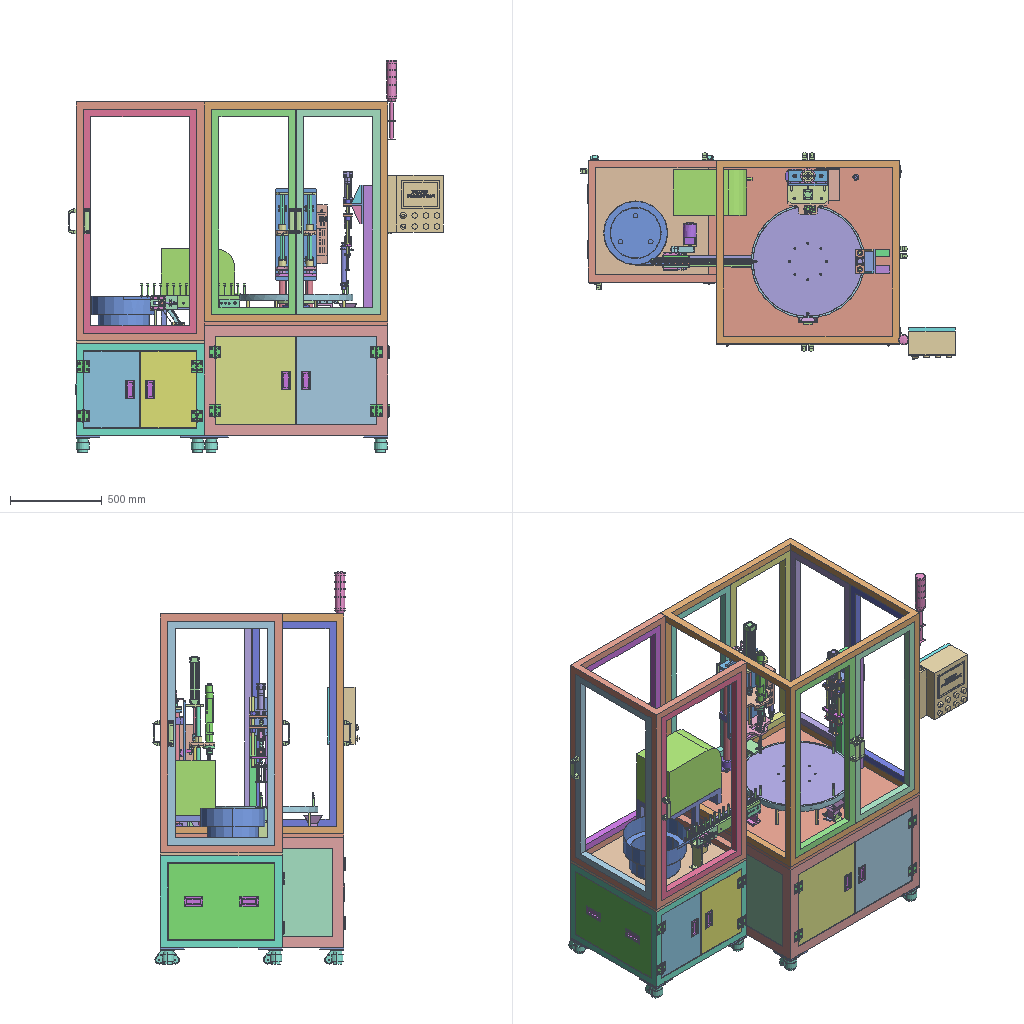Assembly | STEP file | 131 different items | 339 placed | box 2046 x 1125 x 2139 mm
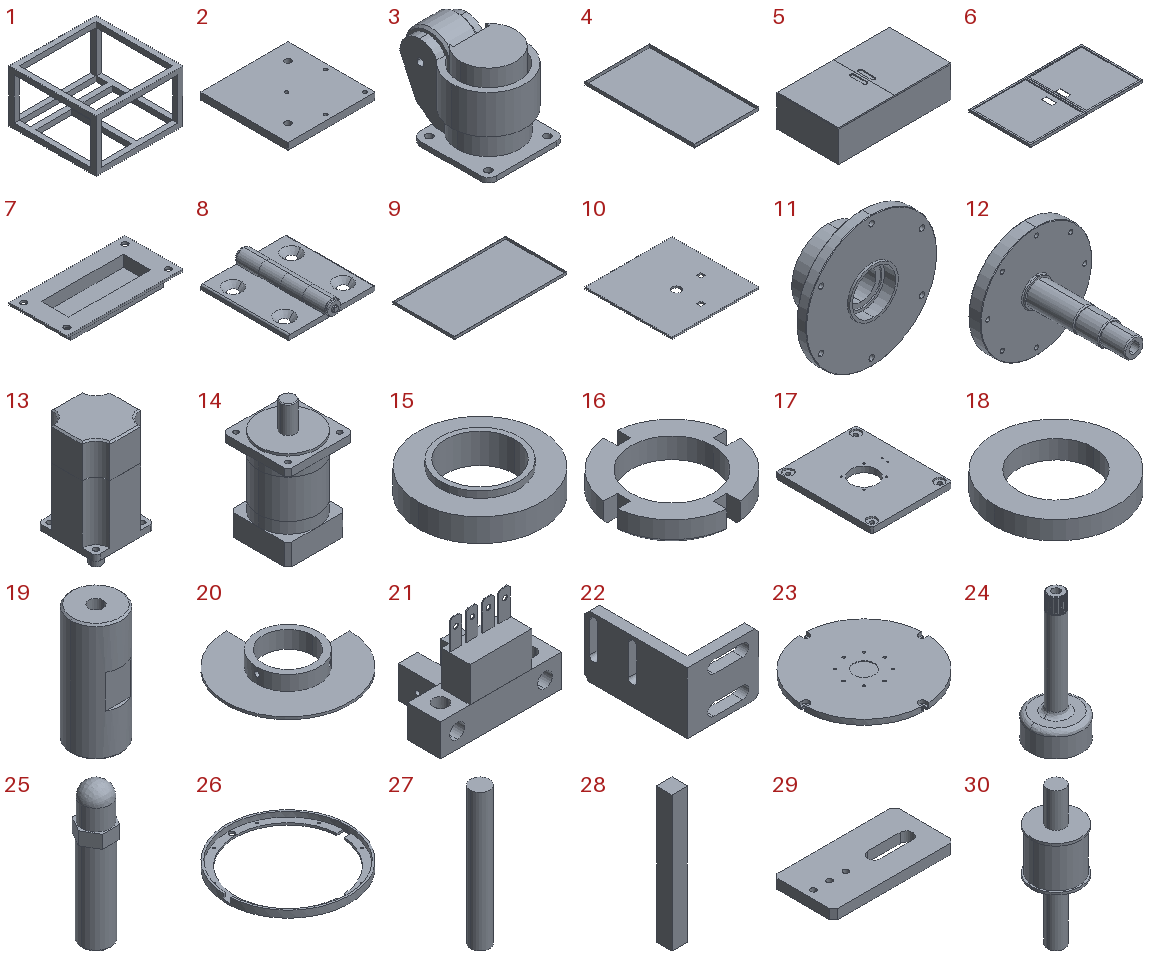Parts list (item | name | quantity | parent item | size | volume):
1 | Lower frame | x1 | in Lower support frame | 1000 x 1000 x 600 mm | 39635953 mm3
2 | Foot plate 2 | x8 | in Lower support frame, Automatic feeding frame | 130 x 130 x 10 mm | 166922 mm3
3 | FM wheel (3 inch) | x8 | in Lower support frame, Automatic feeding frame | 74 x 103.967 x 80 mm | 304180 mm3
4 | Lower sealing plate | x2 | in Lower support frame | 410 x 690 x 20 mm | 485234 mm3
5 | Electrical control box | x1 | in Lower support frame | 880 x 480 x 250 mm | 105113730 mm3
6 | Door | x2 | in Lower support frame | 880 x 480 x 20 mm | 1033932 mm3
7 | Hidden handle | x10 | in Lower support frame, Automatic feeding frame | 102 x 51 x 12.2 mm | 23536 mm3
8 | HHPSN8 hinge | x12 | in Lower support frame, Automatic feeding frame | - | -
9 | Sealing plate | x1 | in Lower support frame | 880 x 480 x 20 mm | 942432 mm3
10 | Large table plate | x1 | in Final assembly | 1000 x 1000 x 20 mm | 19742920 mm3
11 | BB013A02M-04-01A | x1 | in BB013A02M-04-00A | 270 x 95 x 270 mm | 1984635 mm3
12 | BB013A02M-04-02A | x1 | in BB013A02M-04-00A | 230 x 230 x 230 mm | 1390467 mm3
13 | 1FL40-44-0AF21-0AA0 | x1 | in Reducer 2012-6-19 | 80 x 80 x 173 mm | 725829 mm3
14 | PL80-40 | x1 | in Reducer 2012-6-19 | 90 x 90 x 162 mm | 688452 mm3
15 | 30210 | x2 | in BB013A02M-04-00A | 90 x 90 x 21.75 mm | 77564 mm3
16 | M42 nut | x2 | in BB013A02M-04-00A | 71.554 x 71.554 x 12 mm | 23720 mm3
17 | BB013A02M-04-08A | x1 | in BB013A02M-04-00A | 250 x 300 x 18 mm | 1235355 mm3
18 | BB013A02M-04-37A | x1 | in BB013A02M-04-00A | 80 x 80 x 12 mm | 37690 mm3
19 | BB013A02M-04-38A | x4 | in BB013A02M-04-00A | 30 x 30 x 70 mm | 45701 mm3
20 | BB013A02M-04-39A | x1 | in BB013A02M-04-00A | 100 x 100 x 14 mm | 18593 mm3
21 | EE-SX671 (sensing SENSORS) | x1 | in BB013A02M-04-00A | 26.2 x 15.5 x 20.7 mm | 2220 mm3
22 | BB013A02M-04-40A | x1 | in BB013A02M-04-00A | 35 x 50 x 30 mm | 10112 mm3
23 | Turntable | x1 | in Final assembly | 599.815 x 599.815 x 25 mm | 6952769 mm3
24 | Product lower | x20 | in Final assembly, Belt line | 34 x 34 x 83.5 mm | 10000 mm3
25 | Product upper | x3 | in Final assembly | 8.083 x 7 x 31.87 mm | 1117 mm3
26 | Stopper bar | x1 | in Final assembly | 620 x 620 x 35 mm | 1244834 mm3
27 | Support rod | x8 | in Final assembly | 16 x 16 x 114.75 mm | 23072 mm3
28 | Profile | x1 | in Belt line | 40 x 40 x 350 mm | 560000 mm3
29 | Roller fixing plate | x1 | in Belt line | 150 x 75 x 12 mm | 121835 mm3
30 | Driving wheel | x1 | in Belt line | 43 x 43 x 122 mm | 64436 mm3
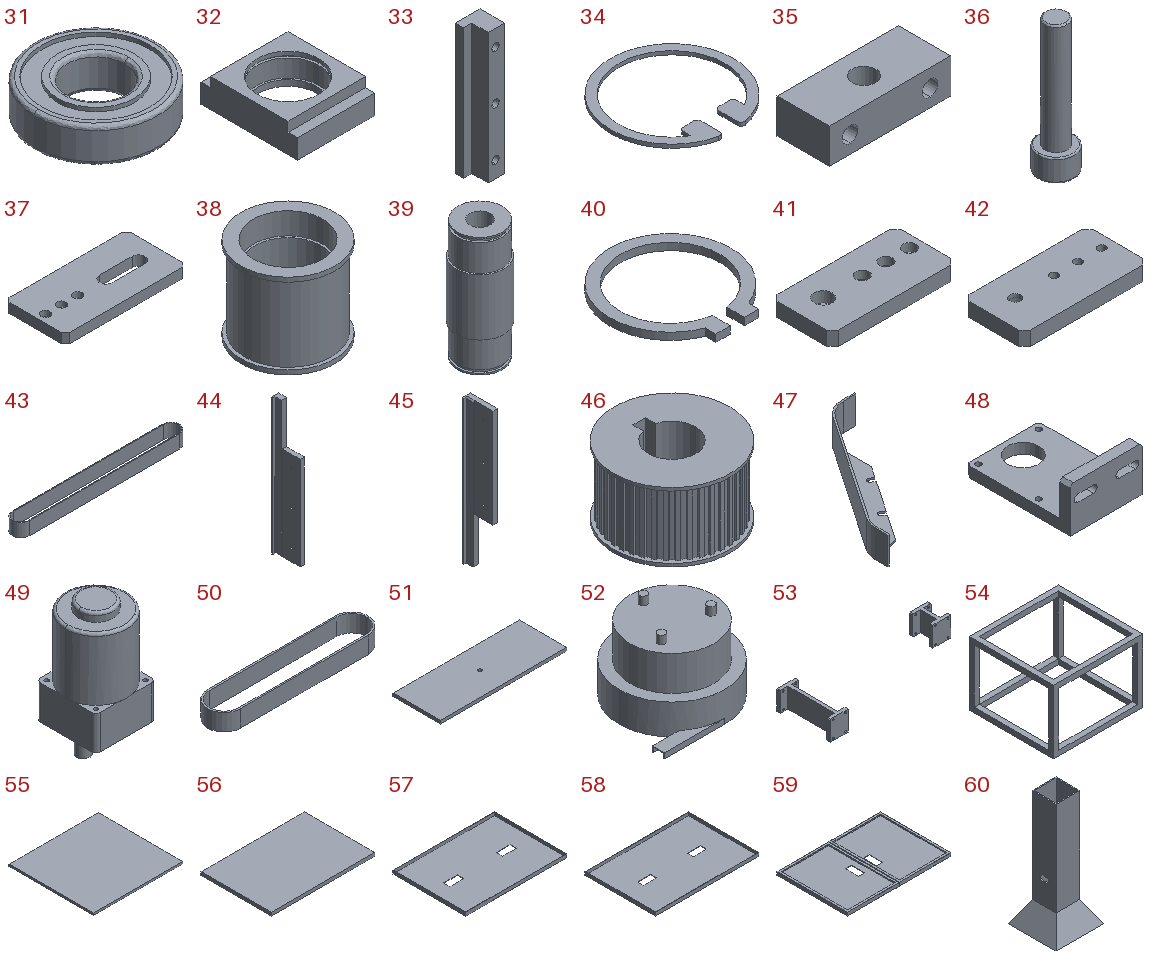31 | 6002 | x4 | in Belt line | 32 x 32 x 9 mm | 4982 mm3
32 | Bearing fixing seat | x2 | in Belt line | 40 x 50 x 15 mm | 16103 mm3
33 | Guide block | x4 | in Belt line | 15 x 15 x 80 mm | 12810 mm3
34 | Inner clip | x2 | in Belt line | 34.4 x 34.017 x 1 mm | 270.275 mm3
35 | Adjusting block | x2 | in Belt line | 35 x 15 x 10 mm | 4094 mm3
36 | Screw | x2 | in Belt line | 13 x 13 x 48 mm | 2788 mm3
37 | Mirror roller fixing plate | x1 | in Belt line | 150 x 75 x 12 mm | 121835 mm3
38 | Driven wheel | x1 | in Belt line | 43 x 43 x 39 mm | 20276 mm3
39 | Driven shaft | x1 | in Belt line | 16 x 16 x 40 mm | 6026 mm3
40 | Outer clip | x2 | in Belt line | 16.8 x 17.727 x 1 mm | 73.853 mm3
41 | Driven wheel fixing plate | x1 | in Belt line | 105 x 52 x 12 mm | 60666 mm3
42 | Mirror driven wheel fixing plate | x1 | in Belt line | 105 x 52 x 12 mm | 60666 mm3
43 | Belt | x1 | in Belt line | 442 x 44 x 35 mm | 64956 mm3
44 | Side stopper bar | x1 | in Belt line | 17.5 x 63 x 335 mm | 183470 mm3
45 | Mirror side stopper bar | x1 | in Belt line | 17.5 x 63 x 335 mm | 183470 mm3
46 | Timing pulley | x2 | in Belt line | 37 x 37 x 22 mm | 16663 mm3
47 | 10020103U05P16_default | x1 | in Belt line | 127 x 167 x 35 mm | 21616 mm3
48 | 10020103U05P11_default | x1 | in Belt line | 70 x 100 x 43 mm | 82196 mm3
49 | M8IA15_default | x1 | in Belt line | 71.8 x 71.8 x 165 mm | 514049 mm3
50 | Timing belt | x1 | in Belt line | 190.16 x 39 x 20 mm | 16742 mm3
51 | Pad plate | x1 | in Belt line | 40 x 15 x 1 mm | 599.215 mm3
52 | Vibratory bowl | x1 | in Belt line | 375 x 350 x 242.5 mm | 663388 mm3
53 | Support plate | x1 | in Belt line | 485 x 170 x 64 mm | 279239 mm3
54 | Small table plate frame | x1 | in Automatic feeding frame | 700 x 665 x 501.75 mm | 10923200 mm3
55 | Small table plate | x1 | in Automatic feeding frame | 700 x 665 x 16 mm | 7448000 mm3
56 | Pad plate 2 | x1 | in Automatic feeding frame | 620 x 420 x 20 mm | 5208000 mm3
57 | Side sealing plate | x1 | in Automatic feeding frame | 585 x 421.75 x 20 mm | 553657 mm3
58 | Rear sealing plate | x1 | in Automatic feeding frame | 620 x 421.75 x 20 mm | 585700 mm3
59 | Side door | x1 | in Automatic feeding frame | 620 x 421.75 x 20 mm | 670167 mm3
60 | Hopper | x2 | in Final assembly | 100 x 100 x 245 mm | 106017 mm3
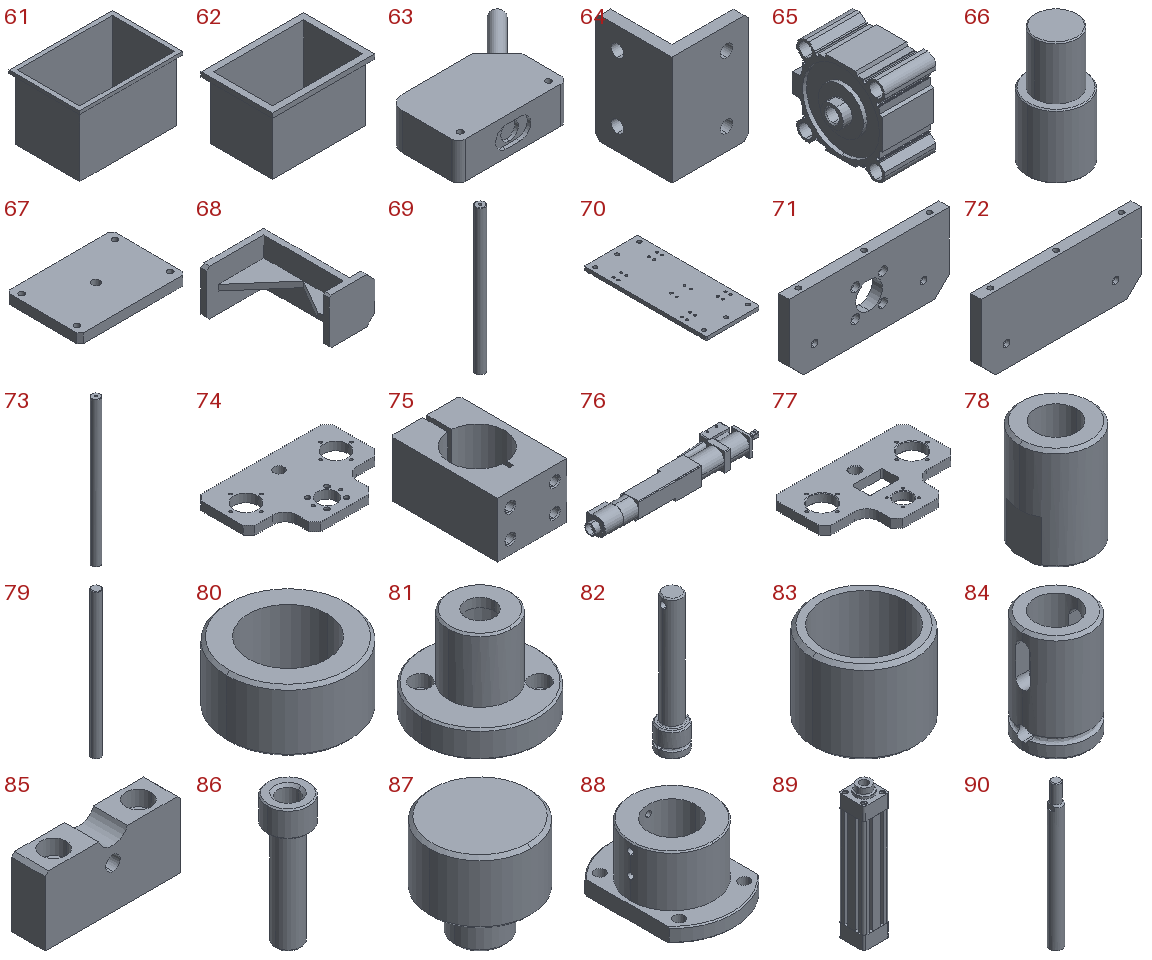61 | Material box | x1 | in Final assembly | 480 x 330 x 300 mm | 3208902 mm3
62 | Material box - copy | x1 | in Final assembly | 330 x 230 x 200 mm | 1493607 mm3
63 | E3Z-T61-L | x4 | in Final assembly | 43.056 x 32.056 x 10.4 mm | 6277 mm3
64 | L bracket | x4 | in Final assembly | 35 x 35 x 50 mm | 15735 mm3
65 | CQ2B100-15DZ(0_0_0) | x1 | in Pressing cylinder | 80 x 123.5 x 117 mm | 628583 mm3
66 | Fixed head | x1 | in Pressing cylinder | 27 x 27 x 55 mm | 25002 mm3
67 | Cylinder pad plate | x1 | in Pressing cylinder | 167 x 117 x 14.75 mm | 282156 mm3
68 | Hook plate | x1 | in Final assembly | 145 x 159.75 x 80 mm | 303088 mm3
69 | fBY02F02M-00-02A | x2 | in fBY02F02M-01-00A | 40 x 40 x 620 mm | 776363 mm3
70 | fBY02F02M-00-04A | x1 | in fBY02F02M-01-00A | 220 x 500 x 14 mm | 1483001 mm3
71 | fBY02F02M-00-08A | x1 | in fBY02F02M-01-00A | 220 x 14 x 100 mm | 276380 mm3
72 | fBY02F02M-00-05A | x1 | in fBY02F02M-01-00A | 220 x 14 x 100 mm | 295677 mm3
73 | fBY02F02M-00-20A | x2 | in fBY02F02M-01-00A | 25 x 25 x 430 mm | 209515 mm3
74 | fBY02F02M-00-07A | x1 | in fBY02F02M-01-00A | 220 x 140 x 14 mm | 291524 mm3
75 | fBY02F02M-00-03A | x4 | in fBY02F02M-01-00A | 50 x 78 x 40 mm | 94734 mm3
76 | fNFT-401RM1A-S | x1 | in fBY02F02M-01-00A | 356.359 x 63.246 x 40.132 mm | 479956 mm3
77 | fBY02F02M-00-06A | x1 | in fBY02F02M-01-00A | 220 x 140 x 14 mm | 261096 mm3
78 | fBY02F02M-00-13A | x1 | in fBY02F02M-01-00A | 25 x 25 x 35 mm | 12210 mm3
79 | fBY02F02M-00-21A | x1 | in fBY02F02M-01-00A | 16 x 16 x 260 mm | 52228 mm3
80 | fBY02F02M-00-19A | x2 | in fBY02F02M-01-00A | 40 x 40 x 20 mm | 14795 mm3
81 | fBY02F02M-00-14A | x1 | in fBY02F02M-02-00A | 65 x 65 x 50 mm | 50405 mm3
82 | fBY02F02M-00-15A | x1 | in fBY02F02M-02-00A | 22 x 22 x 110 mm | 21708 mm3
83 | fBY02F02M-00-16A | x1 | in fBY02F02M-02-00A | 30 x 30 x 24 mm | 7122 mm3
84 | fBY02F02M-00-17A | x1 | in fBY02F02M-02-00A | 24 x 24 x 38 mm | 10216 mm3
85 | fBY02F02M-00-10A | x1 | in fBY02F02M-01-00A | 80 x 20 x 40 mm | 54175 mm3
86 | fBY02F02M-00-11A | x1 | in fBY02F02M-01-00A | 16 x 16 x 50 mm | 4764 mm3
87 | fBY02F02M-00-12A | x1 | in fBY02F02M-01-00A | 16 x 16 x 16 mm | 2297 mm3
88 | fBY02F02M-00-01A | x2 | in fBY02F02M-01-00A | 76 x 104 x 55 mm | 203193 mm3
89 | fA_CP95SB40-150 (0) | x1 | in fcp95sb40-150 | 52 x 52 x 276 mm | 568979 mm3
90 | fA_CP95SB40-150 (0)1 | x1 | in fcp95sb40-150 | 16 x 16 x 188 mm | 35479 mm3
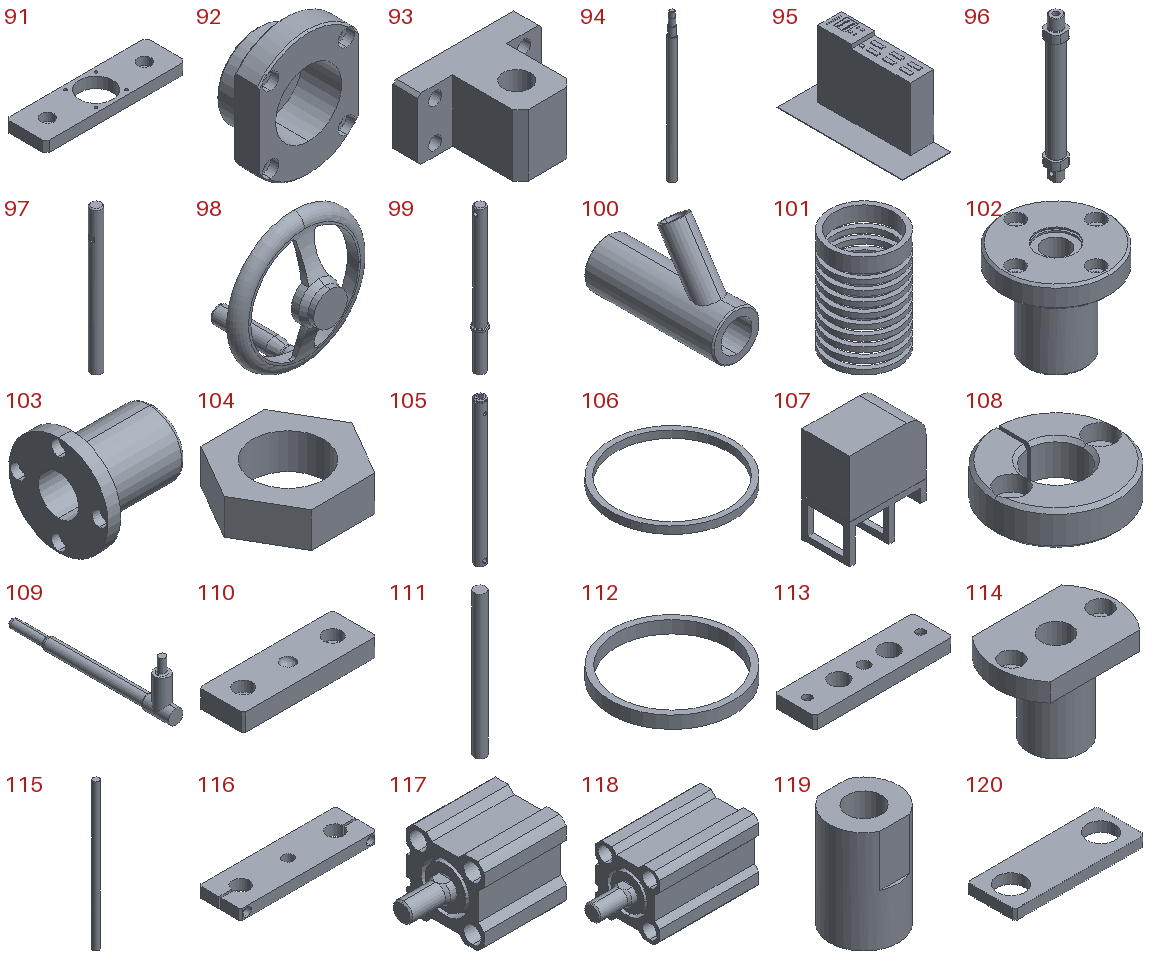91 | fBY02F02M-00-24A | x1 | in fBY02F02M-01-00A | 210 x 60 x 16 mm | 159812 mm3
92 | fBY02F02M-00-25A | x1 | in fBY02F02M-01-00A | 60 x 31 x 75.753 mm | 56251 mm3
93 | fBY02F02M-00-26A | x1 | in fBY02F02M-01-00A | 80 x 60 x 40 mm | 98419 mm3
94 | fBY02F02M-00-27A | x1 | in fBY02F02M-01-00A | 20 x 20 x 409 mm | 120074 mm3
95 | f401kongzhiqi | x1 | in fBY02F02M-01-00A | 122.5 x 320 x 173.5 mm | 2367856 mm3
96 | fA_C85N25-100T(OUT)1 | x1 | in fC85 | 30 x 30 x 257.5 mm | 131255 mm3
97 | fA_C85N25-100T(OUT) | x1 | in fC85 | 10 x 10 x 129 mm | 10086 mm3
98 | fSHLN80 | x1 | in fBY02F02M-01-00A | 80 x 67 x 81.1 mm | 18367 mm3
99 | fBY012F01M-03-01A | x1 | in fBY012F01M-03-00A | 16 x 16 x 172 mm | 18180 mm3
100 | fBY012F01M-03-02A | x1 | in fBY012F01M-03-00A | 18.4 x 50 x 39.602 mm | 7485 mm3
101 | f5-13-063 | x1 | in fBY012F01M-03-00A | 14.1 x 14.1 x 21 mm | 493.858 mm3
102 | fBY02F02M-00-30A | x1 | in fBY02F02M-01-00A | 50 x 50 x 45 mm | 36506 mm3
103 | LHFR-N25 | x4 | in fBY02F02M-01-00A | 59 x 62 x 62 mm | 57510 mm3
104 | M16 nut | x1 | in fBY02F02M-01-00A | 28.868 x 25 x 8 mm | 2722 mm3
105 | Rotating rod | x1 | in fBY02F02M-01-00A | 12 x 12 x 172 mm | 18082 mm3
106 | Extension spring | x25 | in fBY02F02M-01-00A | 17 x 17 x 1 mm | 38.288 mm3
107 | Screw feeder | x1 | in Final assembly | 430 x 250 x 502.25 mm | 31721317 mm3
108 | 08 displacement fixing | x3 | in Displacement detection height | 18 x 17.971 x 5 mm | 899.318 mm3
109 | 08 displacement_default | x1 | in Displacement detection height | 10 x 114.88 x 37 mm | 7298 mm3
110 | Displacement press plate | x1 | in Displacement detection height | 60 x 20 x 8 mm | 8957 mm3
111 | Displacement buffer guide | x2 | in Displacement detection height | 8 x 8 x 100 mm | 5027 mm3
112 | Small spring | x70 | in Displacement detection height | 10 x 10 x 1 mm | 14.923 mm3
113 | Probe fixing plate | x1 | in Displacement detection height | 110 x 32 x 10 mm | 29438 mm3
114 | LMH8UU | x2 | in Displacement detection height | 32 x 21 x 24 mm | 5030 mm3
115 | Guide shaft | x2 | in Displacement detection height | 16 x 16 x 380 mm | 76404 mm3
116 | Cylinder fixing plate 1 | x1 | in Displacement detection height | 130 x 40 x 10 mm | 45360 mm3
117 | CQ2B25-20DM(0_0_0) | x1 | in Displacement detection height | - | -
118 | CQ2B25-40DM(0_0_0) | x1 | in Displacement detection height | - | -
119 | Cylinder joint | x1 | in Displacement detection height | 20 x 20 x 30 mm | 6892 mm3
120 | Linear support fixing plate | x2 | in Displacement detection height | 130 x 48 x 10 mm | 50005 mm3
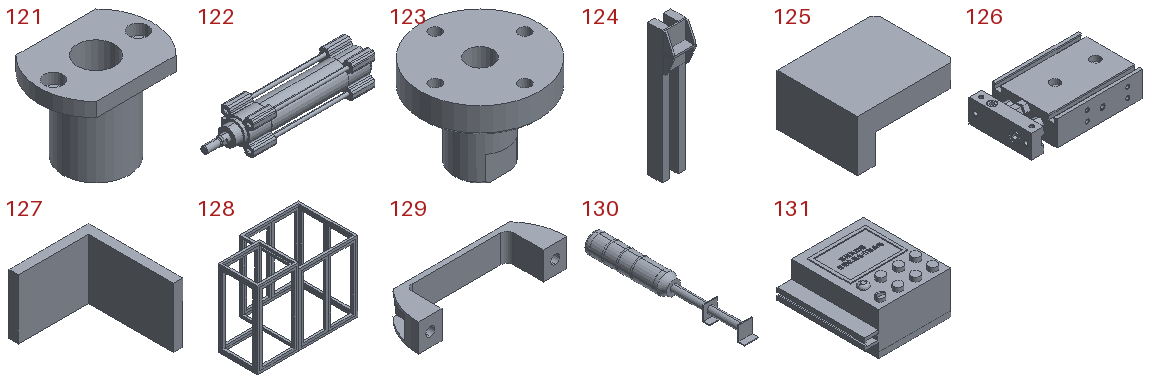121 | LMH16UU | x4 | in Displacement detection height | 48 x 34 x 37 mm | 20039 mm3
122 | C96SB32-80(0_0_0) | x1 | in Displacement detection height | - | -
123 | Connector | x1 | in Displacement detection height | 45 x 45 x 35 mm | 19325 mm3
124 | Connecting plate | x1 | in Displacement detection height | 130 x 142.1 x 745 mm | 5233440 mm3
125 | Cutting plate | x1 | in Cutting mechanism | 44 x 36 x 23 mm | 19544 mm3
126 | CXSM20-35(0_0_0) | x1 | in Cutting mechanism | - | -
127 | Cylinder support plate | x1 | in Cutting mechanism | 85 x 100.75 x 64 mm | 112480 mm3
128 | Upper frame | x1 | in Final assembly | 1700 x 1000 x 1302 mm | 80127840 mm3
129 | UPCN26-B plastic handle | x9 | in Final assembly | 139 x 41 x 26 mm | 36631 mm3
130 | Alarm light 3 | x1 | in Final assembly | 56 x 452 x 56 mm | 602047 mm3
131 | Touch screen 2 | x1 | in Final assembly | 305 x 310 x 172 mm | 12316127 mm3
Placements (level | parent | child | x y z in mm | rotation matrix by rows), first 300 of 352 lines:
1 | Final assembly | Lower support frame | -11.646 -4.778 45.0 | 1 0 0 0 1 0 0 0 1
2 | Lower support frame | Lower frame | -455.325 382.615 -250.0 | 1 0 0 0 1 0 0 0 1
2 | Lower support frame | Foot plate 2 | -452.697 -567.103 -260.0 | 0 1 0 -1 0 0 0 0 1
2 | Lower support frame | Foot plate 2 | -452.697 302.897 -260.0 | 0 1 0 -1 0 0 0 0 1
2 | Lower support frame | Foot plate 2 | 417.303 -567.103 -260.0 | 0 1 0 -1 0 0 0 0 1
2 | Lower support frame | Foot plate 2 | 417.303 302.897 -260.0 | 0 1 0 -1 0 0 0 0 1
2 | Lower support frame | FM wheel (3 inch) | -448.325 -550.385 -260.0 | -1 0 0 0 1 0 0 0 -1
2 | Lower support frame | FM wheel (3 inch) | -448.325 375.615 -260.0 | 1 0 0 0 -1 0 0 0 -1
2 | Lower support frame | FM wheel (3 inch) | 477.675 -550.385 -260.0 | -1 0 0 0 1 0 0 0 -1
2 | Lower support frame | FM wheel (3 inch) | 477.675 375.615 -260.0 | 1 0 0 0 -1 0 0 0 -1
2 | Lower support frame | Lower sealing plate | 249.61 -182.385 -190.0 | -1 0 0 0 1 0 0 0 -1
2 | Lower support frame | Electrical control box | 14.675 162.615 50.0 | 1 0 0 0 0 1 0 -1 0
2 | Lower support frame | Lower sealing plate | -220.33 -182.385 -190.0 | -1 0 0 0 1 0 0 0 -1
2 | Lower support frame | Door | 514.675 -87.385 50.0 | 0 0 -1 -1 0 0 0 1 0
2 | Lower support frame | Hidden handle | 504.475 -32.885 50.0 | 0 0 1 0 1 0 -1 0 0
2 | Lower support frame | Hidden handle | 504.475 -141.885 50.0 | 0 0 1 0 1 0 -1 0 0
2 | Lower support frame | HHPSN8 hinge | 520.175 352.615 205.3 | 0 0 1 -1 0 0 0 -1 0
2 | Lower support frame | HHPSN8 hinge | 520.175 352.615 -114.7 | 0 0 1 -1 0 0 0 -1 0
2 | Lower support frame | HHPSN8 hinge | 520.175 -527.385 205.3 | 0 0 1 -1 0 0 0 -1 0
2 | Lower support frame | HHPSN8 hinge | 520.175 -527.385 -114.7 | 0 0 1 -1 0 0 0 -1 0
2 | Lower support frame | HHPSN8 hinge | 454.675 -592.885 205.3 | -1 0 0 0 0 -1 0 -1 0
2 | Lower support frame | HHPSN8 hinge | 454.675 -592.885 -114.7 | -1 0 0 0 0 -1 0 -1 0
2 | Lower support frame | Hidden handle | 69.175 -577.185 50.0 | 0 1 0 0 0 -1 -1 0 0
2 | Lower support frame | Hidden handle | -39.825 -577.185 50.0 | 0 1 0 0 0 -1 -1 0 0
2 | Lower support frame | HHPSN8 hinge | -425.325 -592.885 -114.7 | -1 0 0 0 0 -1 0 -1 0
2 | Lower support frame | HHPSN8 hinge | -425.325 -592.885 205.3 | -1 0 0 0 0 -1 0 -1 0
2 | Lower support frame | Door | 14.675 -587.385 50.0 | -1 0 0 0 0 1 0 1 0
2 | Lower support frame | Sealing plate | -485.325 -87.385 50.0 | 0 0 1 1 0 0 0 1 0
1 | Final assembly | Large table plate | 3.029 -92.163 395.0 | 1 0 0 0 1 0 0 0 1
1 | Final assembly | BB013A02M-04-00A | 344.4 -189.063 134.949 | 1 0 0 0 1 0 0 0 1
2 | BB013A02M-04-00A | BB013A02M-04-01A | -341.371 46.9 211.718 | 0.9983 0 0.05751 0.05751 0 -0.9983 0 1 0
2 | BB013A02M-04-00A | BB013A02M-04-02A | -341.371 46.9 172.801 | 1 0 0 0 0 -1 0 1 0
2 | BB013A02M-04-00A | Reducer 2012-6-19 | -343.105 58.644 3.551 | 0 1 0 1 0 0 0 0 -1
3 | Reducer 2012-6-19 | 1FL40-44-0AF21-0AA0 | -11.745 1.734 -46.5 | 1 0 0 0 1 0 0 0 1
3 | Reducer 2012-6-19 | PL80-40 | -11.745 1.734 -46.5 | 1 0 0 0 -1 0 0 0 -1
2 | BB013A02M-04-00A | 30210 | -341.371 46.9 353.051 | 1 0 0 0 1 0 0 0 1
2 | BB013A02M-04-00A | 30210 | -341.371 46.9 298.051 | -0.9237 -0.383 0 -0.383 0.9237 0 0 0 -1
2 | BB013A02M-04-00A | M42 nut | -341.371 46.9 252.301 | 0.9998 0.01986 0 -0.01986 0.9998 0 0 0 1
2 | BB013A02M-04-00A | M42 nut | -341.371 46.9 240.301 | 0.9998 0.01986 0 -0.01986 0.9998 0 0 0 1
2 | BB013A02M-04-00A | BB013A02M-04-08A | -341.371 46.9 172.051 | 1 0 0 0 1 0 0 0 1
2 | BB013A02M-04-00A | BB013A02M-04-37A | -341.371 46.9 264.301 | 1 0 0 0 1 0 0 0 1
2 | BB013A02M-04-00A | BB013A02M-04-38A | -446.371 -83.1 260.051 | -0.9237 -0.383 0 -0.383 0.9237 0 0 0 -1
2 | BB013A02M-04-00A | BB013A02M-04-38A | -446.371 176.899 260.051 | -0.9237 -0.383 0 -0.383 0.9237 0 0 0 -1
2 | BB013A02M-04-00A | BB013A02M-04-38A | -236.371 -83.1 260.051 | -0.9237 -0.383 0 -0.383 0.9237 0 0 0 -1
2 | BB013A02M-04-00A | BB013A02M-04-38A | -236.371 176.899 260.051 | -0.9237 -0.383 0 -0.383 0.9237 0 0 0 -1
2 | BB013A02M-04-00A | BB013A02M-04-39A | -341.371 46.9 227.801 | 1 0 0 0 -1 0 0 0 -1
2 | BB013A02M-04-00A | EE-SX671 (sensing SENSORS) | -281.371 47.374 226.301 | 0 -1 0 0 0 1 -1 0 0
2 | BB013A02M-04-00A | BB013A02M-04-40A | -281.371 73.9 240.051 | 1 0 0 0 0 -1 0 1 0
1 | Final assembly | Turntable | 3.029 -142.163 564.75 | -1 0 0 0 1 0 0 0 -1
1 | Final assembly | Product lower | 3.029 -425.163 539.75 | 0 -1 0 1 0 0 0 0 1
1 | Final assembly | Product lower | -279.971 -142.163 539.75 | 1 0 0 0 1 0 0 0 1
1 | Final assembly | Product lower | 3.029 140.837 539.75 | 0 1 0 -1 0 0 0 0 1
1 | Final assembly | Product lower | 286.029 -142.163 539.75 | -1 0 0 0 -1 0 0 0 1
1 | Final assembly | Product upper | 3.029 140.837 632.25 | 1 0 0 0 1 0 0 0 1
1 | Final assembly | Product upper | 286.029 -142.163 632.25 | 0 1 0 -1 0 0 0 0 1
1 | Final assembly | Product upper | 3.029 -425.163 632.25 | -1 0 0 0 -1 0 0 0 1
1 | Final assembly | Stopper bar | 3.029 -142.163 529.75 | 1 0 0 0 1 0 0 0 1
1 | Final assembly | Support rod | -260.203 -33.129 415.0 | 1 0 0 0 1 0 0 0 1
1 | Final assembly | Support rod | -260.203 -251.197 415.0 | 0.7071 -0.7071 0 0.7071 0.7071 0 0 0 1
1 | Final assembly | Support rod | -106.005 -405.395 415.0 | 0 -1 0 1 0 0 0 0 1
1 | Final assembly | Support rod | 112.063 -405.395 415.0 | -0.7071 -0.7071 0 0.7071 -0.7071 0 0 0 1
1 | Final assembly | Support rod | 266.261 -251.197 415.0 | -1 0 0 0 -1 0 0 0 1
1 | Final assembly | Support rod | 266.261 -33.129 415.0 | -0.7071 0.7071 0 -0.7071 -0.7071 0 0 0 1
1 | Final assembly | Support rod | 112.063 121.069 415.0 | 0 1 0 -1 0 0 0 0 1
1 | Final assembly | Support rod | -106.005 121.069 415.0 | 0.7071 0.7071 0 -0.7071 0.7071 0 0 0 1
1 | Final assembly | Belt line | -601.971 -91.057 499.385 | 0 0 -1 -1 0 0 0 1 0
2 | Belt line | Profile | 51.106 18.365 -250.0 | 1 0 0 0 1 0 0 0 1
2 | Belt line | Roller fixing plate | 83.106 20.865 115.0 | 0 0 -1 0 1 0 1 0 -0
2 | Belt line | Driving wheel | 33.606 18.365 125.0 | 0 0 1 0.7219 0.692 0 -0.692 0.7219 0
2 | Belt line | 6002 | 95.106 18.365 125.0 | 0 0 -1 -0.5396 0.8419 0 0.8419 0.5396 0
2 | Belt line | Bearing fixing seat | 83.106 18.365 125.0 | 0 0 1 0 1 0 -1 0 0
2 | Belt line | Guide block | 93.106 -1.635 105.0 | 0 1 0 -1 0 0 0 0 1
2 | Belt line | Guide block | 93.106 38.365 185.0 | 0 1 0 1 0 0 0 0 -1
2 | Belt line | Inner clip | 96.106 18.365 125.0 | 0 0 -1 0 1 0 1 0 -0
2 | Belt line | Adjusting block | 90.606 18.365 75.0 | 0 1 0 -1 0 0 0 0 1
2 | Belt line | Screw | 90.606 18.365 57.0 | 1 0 0 0 1 0 0 0 1
2 | Belt line | Mirror roller fixing plate | 19.106 20.865 115.0 | 0 0 -1 0 1 0 1 0 -0
2 | Belt line | Guide block | 9.106 38.365 105.0 | 0 -1 0 1 0 0 0 0 1
2 | Belt line | Bearing fixing seat | 19.106 18.365 125.0 | 0 0 -1 0 1 0 1 0 0
2 | Belt line | 6002 | 7.106 18.365 125.0 | 0 0 1 0.5396 0.8419 0 -0.8419 0.5396 0
2 | Belt line | Inner clip | 7.106 18.365 125.0 | 0 0 -1 0 1 0 1 0 0
2 | Belt line | Screw | 11.606 18.365 57.0 | 1 0 0 0 1 0 0 0 1
2 | Belt line | Adjusting block | 11.606 18.365 75.0 | 0 -1 0 1 0 0 0 0 1
2 | Belt line | Guide block | 9.106 -1.635 185.0 | 0 -1 0 -1 0 0 0 0 -1
2 | Belt line | Driven wheel | 68.606 18.365 -273.0 | 0 0 -1 0 1 0 1 0 0
2 | Belt line | 6002 | 69.606 18.365 -273.0 | 0 0 -1 0 1 0 1 0 0
2 | Belt line | 6002 | 41.606 18.365 -273.0 | 0 0 -1 0 1 0 1 0 0
2 | Belt line | Driven shaft | 60.606 18.365 -273.0 | 0 0 -1 0 1 0 1 0 0
2 | Belt line | Outer clip | 70.606 18.365 -273.0 | 0 0 -1 0 1 0 1 0 0
2 | Belt line | Outer clip | 32.606 18.365 -273.0 | 0 0 -1 0 1 0 1 0 0
2 | Belt line | Driven wheel fixing plate | 31.106 23.365 -242.5 | 0 0 -1 0 1 0 1 0 -0
2 | Belt line | Mirror driven wheel fixing plate | 71.106 23.365 -242.5 | 0 0 -1 0 1 0 1 0 -0
2 | Belt line | Belt | 68.606 18.365 -273.0 | 0 0 -1 0 1 0 1 0 -0
2 | Belt line | Side stopper bar | 31.106 -3.635 40.0 | -1 0 0 0 1 0 0 0 -1
2 | Belt line | Mirror side stopper bar | 71.106 -3.635 40.0 | 1 0 0 0 1 0 0 0 1
2 | Belt line | Timing pulley | -19.894 18.365 125.0 | 0 0 1 0 1 0 -1 0 0
2 | Belt line | 10020103U05P16_default | 2.106 18.365 125.0 | 0 0 -1 0 1 0 1 0 -0
2 | Belt line | Timing pulley | 0.1063 -106.635 40.0 | 0 0 -1 0 1 0 1 0 -0
2 | Belt line | 10020103U05P11_default | -30.894 -136.635 40.0 | 0 0 -1 0 1 0 1 0 -0
2 | Belt line | M8IA15_default | -40.894 -121.635 40.0 | 0 0 -1 0 1 0 1 0 0
2 | Belt line | Timing belt | -19.894 18.365 125.0 | 0 0 1 -0.8269 0.5623 0 -0.5623 -0.8269 0
2 | Belt line | Pad plate | 51.106 40.365 -287.5 | 1 0 0 0 0 -1 0 1 0
2 | Belt line | Product lower | 51.106 40.365 -287.5 | 1 0 0 0 0 1 0 -1 0
2 | Belt line | Product lower | 51.106 40.365 -252.5 | 1 0 0 0 0 1 0 -1 0
2 | Belt line | Product lower | 51.106 40.365 -217.5 | 1 0 0 0 0 1 0 -1 0
2 | Belt line | Product lower | 51.106 40.365 -182.5 | 1 0 0 0 0 1 0 -1 0
2 | Belt line | Product lower | 51.106 40.365 -147.5 | 1 0 0 0 0 1 0 -1 0
2 | Belt line | Product lower | 51.106 40.365 -112.5 | 1 0 0 0 0 1 0 -1 0
2 | Belt line | Product lower | 51.106 40.365 -77.5 | 1 0 0 0 0 1 0 -1 0
2 | Belt line | Product lower | 51.106 40.365 -42.5 | 1 0 0 0 0 1 0 -1 0
2 | Belt line | Product lower | 51.106 40.365 -7.5 | 1 0 0 0 0 1 0 -1 0
2 | Belt line | Product lower | 51.106 40.365 27.5 | 1 0 0 0 0 1 0 -1 0
2 | Belt line | Product lower | 51.106 40.365 62.5 | 1 0 0 0 0 1 0 -1 0
2 | Belt line | Product lower | 51.106 40.365 97.5 | 1 0 0 0 0 1 0 -1 0
2 | Belt line | Product lower | 51.106 40.365 132.5 | 1 0 0 0 0 1 0 -1 0
2 | Belt line | Vibratory bowl | -103.894 55.865 335.0 | 0 -1 0 0 0 -1 1 0 -0
2 | Belt line | Product lower | 51.106 40.365 167.5 | 1 0 0 0 0 1 0 -1 0
2 | Belt line | Product lower | 51.106 40.365 202.5 | 1 0 0 0 0 1 0 -1 0
2 | Belt line | Product lower | 51.106 40.365 237.5 | 1 0 0 0 0 1 0 -1 0
2 | Belt line | Support plate | 19.106 -11.635 190.0 | 0 0 1 0 1 0 -1 0 0
1 | Final assembly | Automatic feeding frame | -852.986 77.278 45.875 | 1 0 0 0 1 0 0 0 1
2 | Automatic feeding frame | Small table plate frame | 6.015 -1.941 -250.875 | 1 0 0 0 1 0 0 0 1
2 | Automatic feeding frame | Small table plate | 6.015 -1.941 250.875 | 1 0 0 0 1 0 0 0 1
2 | Automatic feeding frame | Foot plate 2 | -311.357 -314.159 -260.875 | 0 1 0 -1 0 0 0 0 1
2 | Automatic feeding frame | Foot plate 2 | -311.357 220.841 -260.875 | 0 1 0 -1 0 0 0 0 1
2 | Automatic feeding frame | Foot plate 2 | 258.643 -314.159 -260.875 | 0 1 0 -1 0 0 0 0 1
2 | Automatic feeding frame | Foot plate 2 | 258.643 220.841 -260.875 | 0 1 0 -1 0 0 0 0 1
2 | Automatic feeding frame | FM wheel (3 inch) | -306.985 -297.441 -260.875 | -1 0 0 0 1 0 0 0 -1
2 | Automatic feeding frame | FM wheel (3 inch) | -306.985 293.559 -260.875 | -1 0 0 0 1 0 0 0 -1
2 | Automatic feeding frame | FM wheel (3 inch) | 319.015 -297.441 -260.875 | -1 0 0 0 1 0 0 0 -1
2 | Automatic feeding frame | FM wheel (3 inch) | 319.015 293.559 -260.875 | -1 0 0 0 1 0 0 0 -1
2 | Automatic feeding frame | Pad plate 2 | 6.015 80.559 -230.875 | 1 0 0 0 1 0 0 0 1
2 | Automatic feeding frame | Side sealing plate | -343.985 -1.941 -0.0 | 0 0 1 1 0 0 0 1 0
2 | Automatic feeding frame | Hidden handle | -333.785 150.059 -0.0 | 0 0 -1 -1 0 0 0 1 -0
2 | Automatic feeding frame | Rear sealing plate | 6.015 330.559 0.0 | 1 0 0 0 0 -1 0 1 0
2 | Automatic feeding frame | Hidden handle | 155.515 320.359 0.0 | 1 0 0 0 0 1 0 -1 0
2 | Automatic feeding frame | Hidden handle | -143.485 320.359 0.0 | 1 0 0 0 0 1 0 -1 0
2 | Automatic feeding frame | Side door | 6.015 -334.441 -0.0 | 1 0 0 0 0 1 0 -1 0
2 | Automatic feeding frame | Hidden handle | 60.515 -324.241 0.0 | 0 -1 0 0 0 -1 1 0 0
2 | Automatic feeding frame | Hidden handle | -48.485 -324.241 0.0 | 0 -1 0 0 0 -1 1 0 0
2 | Automatic feeding frame | HHPSN8 hinge | 316.015 -339.941 126.175 | 1 0 0 0 0 -1 0 1 0
2 | Automatic feeding frame | HHPSN8 hinge | 316.015 -339.941 -143.825 | 1 0 0 0 0 -1 0 1 0
2 | Automatic feeding frame | HHPSN8 hinge | -303.985 -339.941 126.175 | 1 0 0 0 0 -1 0 1 0
2 | Automatic feeding frame | HHPSN8 hinge | -303.985 -339.941 -143.825 | 1 0 0 0 0 -1 0 1 0
2 | Automatic feeding frame | Hidden handle | -333.785 -153.941 -0.0 | 0 0 -1 -1 0 0 0 1 -0
1 | Final assembly | Hopper | 3.029 -425.163 514.75 | -1 0 0 0 1 0 0 0 -1
1 | Final assembly | Hopper | 286.029 -142.163 514.75 | 0 -1 0 -1 0 0 0 0 -1
1 | Final assembly | Material box | -36.971 -390.163 -145.0 | 1 0 0 0 1 0 0 0 1
1 | Final assembly | Material box - copy | 306.029 -142.163 -145.0 | 0 -1 0 1 0 0 0 0 1
1 | Final assembly | E3Z-T61-L | -21.971 -442.163 415.0 | 0 -1 0 1 0 0 0 0 1
1 | Final assembly | E3Z-T61-L | 28.029 -442.163 425.4 | 0 1 0 1 0 0 0 0 -1
1 | Final assembly | E3Z-T61-L | 303.029 -117.163 425.4 | -1 0 0 0 1 0 0 0 -1
1 | Final assembly | E3Z-T61-L | 303.029 -167.163 415.0 | -1 0 0 0 -1 0 0 0 1
1 | Final assembly | L bracket | 28.029 -450.163 450.0 | 0 0 -1 -1 0 0 0 1 0
1 | Final assembly | L bracket | -21.971 -400.163 450.0 | 0 0 1 1 0 0 0 1 0
1 | Final assembly | L bracket | 261.029 -167.163 450.0 | -1 0 0 0 0 1 0 1 0
1 | Final assembly | L bracket | 311.029 -117.163 450.0 | 1 0 0 0 0 -1 0 1 0
1 | Final assembly | Pressing cylinder | 22.325 140.837 460.834 | 0 -1 0 0 0 1 -1 0 0
2 | Pressing cylinder | CQ2B100-15DZ(0_0_0) | -36.916 19.296 -0.0 | 1 0 0 0 1 0 0 0 1
2 | Pressing cylinder | Fixed head | -78.916 19.296 0.0 | 0 0 1 0 1 0 -1 0 -0
2 | Pressing cylinder | Cylinder pad plate | 45.834 19.296 -0.0 | 0 0 -1 -1 0 0 0 1 0
1 | Final assembly | Hook plate | -36.971 147.837 564.75 | 0 0 1 1 0 0 0 1 -0
1 | Final assembly | fBY02F02M-01-00A | -179.249 533.293 824.53 | 0 1 -0.000385 -1 0 0 0 0.000385 1
2 | fBY02F02M-01-00A | fBY02F02M-00-02A | 210.454 109.802 -397.719 | 0.4882 -0.8727 0 0.8727 0.4882 0 0 0 1
2 | fBY02F02M-01-00A | fBY02F02M-00-02A | 210.454 254.802 -397.719 | 0.9253 0.3793 0 -0.3793 0.9253 0 0 0 1
2 | fBY02F02M-01-00A | fBY02F02M-00-04A | 264.454 292.302 318.281 | 0 0 -1 -1 0 0 0 1 0
2 | fBY02F02M-01-00A | fBY02F02M-00-08A | 362.454 292.302 298.281 | 0 0 -1 -1 0 0 0 1 0
2 | fBY02F02M-01-00A | fBY02F02M-00-05A | 362.454 292.302 -145.719 | 0 0 -1 -1 0 0 0 1 0
2 | fBY02F02M-01-00A | fBY02F02M-00-20A | 332.454 107.302 -145.719 | 1 0 0 0 1 0 0 0 1
2 | fBY02F02M-01-00A | fBY02F02M-00-20A | 332.454 257.302 -145.719 | 0.9995 0.03267 0 -0.03267 0.9995 0 0 0 1
2 | fBY02F02M-01-00A | fBY02F02M-00-07A | 282.454 292.302 86.584 | 0 -1 0 -1 0 0 0 0 -1
2 | fBY02F02M-01-00A | fBY02F02M-00-03A | 250.454 254.802 -71.719 | 0 -1 0 1 0 0 0 0 1
2 | fBY02F02M-01-00A | fBY02F02M-00-03A | 250.454 254.802 208.281 | 0 -1 0 1 0 0 0 0 1
2 | fBY02F02M-01-00A | fNFT-401RM1A-S | 392.454 182.302 86.584 | 0 0 1 0 1 0 -1 0 0
2 | fBY02F02M-01-00A | fBY02F02M-00-06A | 282.454 72.302 -121.416 | 0 -1 0 1 0 0 0 0 1
2 | fBY02F02M-01-00A | fBY02F02M-00-13A | 312.454 182.302 98.584 | 1 0 0 0 1 0 0 0 1
2 | fBY02F02M-01-00A | fBY02F02M-00-21A | 312.454 182.302 -141.416 | -0.9817 0.1903 0 -0.1903 -0.9817 0 0 0 1
2 | fBY02F02M-01-00A | fBY02F02M-00-19A | 332.454 107.302 -145.719 | 1 0 0 0 1 0 0 0 1
2 | fBY02F02M-01-00A | fBY02F02M-00-19A | 332.454 257.302 -145.719 | 1 0 0 0 1 0 0 0 1
2 | fBY02F02M-01-00A | fBY02F02M-02-00A | 386.507 173.884 65.584 | 0.7071 0.7071 0 0.7071 -0.7071 0 0 0 -1
3 | fBY02F02M-02-00A | fBY02F02M-00-14A | 10.157 -1.747 -7 | 1 0 0 0 1 0 0 0 1
3 | fBY02F02M-02-00A | fBY02F02M-00-15A | 10.161 -1.747 -2.71 | 0.7071 -0.7071 -0.000272 0.7071 0.7071 0.000272 0 -0.000385 1
3 | fBY02F02M-02-00A | fBY02F02M-00-16A | 10.135 -1.722 90.29 | -0.3615 0.9324 -0.000272 -0.9324 -0.3615 0.000272 0.000155 0.000352 1
3 | fBY02F02M-02-00A | fBY02F02M-00-17A | 10.124 -1.71 133.29 | -0.7071 -0.7071 0.000272 -0.7071 0.7071 -0.000272 0 -0.000385 -1
2 | fBY02F02M-01-00A | fBY02F02M-00-10A | 264.454 222.302 33.281 | 0 0 1 -1 0 0 0 -1 -0
2 | fBY02F02M-01-00A | fBY02F02M-00-11A | 289.454 182.302 23.281 | 0.8148 0.5797 0 -0.5797 0.8148 0 0 0 1
2 | fBY02F02M-01-00A | fBY02F02M-00-12A | 289.454 182.302 67.281 | 1 0 0 0 1 0 0 0 1
2 | fBY02F02M-01-00A | fBY02F02M-00-01A | 210.454 109.802 -409.642 | 1 0 0 0 1 0 0 0 1
2 | fBY02F02M-01-00A | fBY02F02M-00-01A | 210.454 254.802 -409.642 | 1 0 0 0 1 0 0 0 1
2 | fBY02F02M-01-00A | fBY02F02M-00-03A | 250.454 109.802 -71.719 | 0 -1 0 1 0 0 0 0 1
2 | fBY02F02M-01-00A | fBY02F02M-00-03A | 250.454 109.802 208.281 | 0 -1 0 1 0 0 0 0 1
2 | fBY02F02M-01-00A | fcp95sb40-150 | 307.391 169.305 419.281 | -1 0 0 0 1 0 0 0 -1
3 | fcp95sb40-150 | fA_CP95SB40-150 (0) | -5.062 12.997 121.0 | 1 0 0 0 1 0 0 0 1
3 | fcp95sb40-150 | fA_CP95SB40-150 (0)1 | -5.062 12.997 251.698 | -0.7861 0.6181 0 -0.6181 -0.7861 0 0 0 1
2 | fBY02F02M-01-00A | fBY02F02M-00-24A | 240.454 287.302 252.281 | 0 1 0 -1 0 0 0 0 1
2 | fBY02F02M-01-00A | fBY02F02M-00-25A | 210.454 182.302 252.281 | -1 0 0 0 0 -1 0 -1 0
2 | fBY02F02M-01-00A | fBY02F02M-00-26A | 250.454 222.302 12.281 | 0 1 0 -1 0 0 0 0 1
2 | fBY02F02M-01-00A | fBY02F02M-00-27A | 210.454 182.302 -90.719 | 0.7507 -0.6606 0 0.6606 0.7507 0 0 0 1
2 | fBY02F02M-01-00A | f401kongzhiqi | 172.454 292.302 186.944 | 0 0 1 1 0 0 0 1 -0
2 | fBY02F02M-01-00A | fC85 | 195.23 443.42 -105.892 | -0.5199 0.8542 0 0.8542 0.5199 0 0 0 -1
3 | fC85 | fA_C85N25-100T(OUT)1 | -11.797 18.687 128.75 | 1 0 0 0 1 0 0 0 1
3 | fC85 | fA_C85N25-100T(OUT) | -11.797 18.687 23.003 | -0.235 -0.972 0 0.972 -0.235 0 0 0 1
2 | fBY02F02M-01-00A | fSHLN80 | 210.454 182.302 306.581 | 1 0 0 0 0 -1 0 1 0
2 | fBY02F02M-01-00A | fBY012F01M-03-00A | 396.052 182.16 154.359 | 1 0 0 0 0.000385 -1 0 1 0.000385
3 | fBY012F01M-03-00A | fBY012F01M-03-01A | -3.596 -380.565 -0.178 | -1 0 0 0 0 1 0 1 -0
3 | fBY012F01M-03-00A | fBY012F01M-03-02A | -3.596 -399.065 -0.178 | 1 0 0 0 1 0 0 0 1
3 | fBY012F01M-03-00A | f5-13-063 | -3.596 -336.065 -0.178 | 0.72 0.694 0 0 0 -1 -0.694 0.72 0
2 | fBY02F02M-01-00A | fBY02F02M-00-30A | 392.454 182.302 -142.416 | 0.7071 0.7071 0 -0.7071 0.7071 0 0 0 1
2 | fBY02F02M-01-00A | LHFR-N25 | 332.454 107.302 64.584 | 0 1 0 0 0 1 1 0 0
2 | fBY02F02M-01-00A | LHFR-N25 | 332.454 257.302 64.584 | 0 1 0 0 0 1 1 0 0
2 | fBY02F02M-01-00A | LHFR-N25 | 332.454 107.302 -129.416 | 0 1 0 0 0 1 1 0 -0
2 | fBY02F02M-01-00A | LHFR-N25 | 332.454 257.302 -129.416 | 0 1 0 0 0 1 1 0 -0
2 | fBY02F02M-01-00A | M16 nut | 312.454 182.302 -129.416 | 0 1 0 -1 0 0 0 0 1
2 | fBY02F02M-01-00A | Rotating rod | 392.456 182.257 -55.707 | 0 1 0 1 0 -0.000385 -0.000385 0 -1
2 | fBY02F02M-01-00A | Extension spring | 392.456 182.267 -28.707 | -1 -4.4e-05 0 4.4e-05 -1 0.000385 0 0.000385 1
2 | fBY02F02M-01-00A | Extension spring | 392.456 182.267 -26.707 | -1 -4.4e-05 0 4.4e-05 -1 0.000385 0 0.000385 1
2 | fBY02F02M-01-00A | Extension spring | 392.456 182.267 -24.707 | -1 -4.4e-05 0 4.4e-05 -1 0.000385 0 0.000385 1
2 | fBY02F02M-01-00A | Extension spring | 392.456 182.267 -22.707 | -1 -4.4e-05 0 4.4e-05 -1 0.000385 0 0.000385 1
2 | fBY02F02M-01-00A | Extension spring | 392.456 182.267 -20.707 | -1 -4.4e-05 0 4.4e-05 -1 0.000385 0 0.000385 1
2 | fBY02F02M-01-00A | Extension spring | 392.456 182.267 -18.707 | -1 -4.4e-05 0 4.4e-05 -1 0.000385 0 0.000385 1
2 | fBY02F02M-01-00A | Extension spring | 392.456 182.267 -16.707 | -1 -4.4e-05 0 4.4e-05 -1 0.000385 0 0.000385 1
2 | fBY02F02M-01-00A | Extension spring | 392.456 182.267 -14.707 | -1 -4.4e-05 0 4.4e-05 -1 0.000385 0 0.000385 1
2 | fBY02F02M-01-00A | Extension spring | 392.456 182.267 -12.707 | -1 -4.4e-05 0 4.4e-05 -1 0.000385 0 0.000385 1
2 | fBY02F02M-01-00A | Extension spring | 392.456 182.267 -10.707 | -1 -4.4e-05 0 4.4e-05 -1 0.000385 0 0.000385 1
2 | fBY02F02M-01-00A | Extension spring | 392.456 182.267 -8.707 | -1 -4.4e-05 0 4.4e-05 -1 0.000385 0 0.000385 1
2 | fBY02F02M-01-00A | Extension spring | 392.456 182.267 -6.707 | -1 -4.4e-05 0 4.4e-05 -1 0.000385 0 0.000385 1
2 | fBY02F02M-01-00A | Extension spring | 392.456 182.267 -4.707 | -1 -4.4e-05 0 4.4e-05 -1 0.000385 0 0.000385 1
2 | fBY02F02M-01-00A | Extension spring | 392.456 182.267 -2.707 | -1 -4.4e-05 0 4.4e-05 -1 0.000385 0 0.000385 1
2 | fBY02F02M-01-00A | Extension spring | 392.456 182.267 -0.7068 | -1 -4.4e-05 0 4.4e-05 -1 0.000385 0 0.000385 1
2 | fBY02F02M-01-00A | Extension spring | 392.456 182.267 1.293 | -1 -4.4e-05 0 4.4e-05 -1 0.000385 0 0.000385 1
2 | fBY02F02M-01-00A | Extension spring | 392.456 182.267 3.293 | -1 -4.4e-05 0 4.4e-05 -1 0.000385 0 0.000385 1
2 | fBY02F02M-01-00A | Extension spring | 392.456 182.267 5.293 | -1 -4.4e-05 0 4.4e-05 -1 0.000385 0 0.000385 1
2 | fBY02F02M-01-00A | Extension spring | 392.456 182.267 7.293 | -1 -4.4e-05 0 4.4e-05 -1 0.000385 0 0.000385 1
2 | fBY02F02M-01-00A | Extension spring | 392.456 182.267 9.293 | -1 -4.4e-05 0 4.4e-05 -1 0.000385 0 0.000385 1
2 | fBY02F02M-01-00A | Extension spring | 392.456 182.267 11.293 | -1 -4.4e-05 0 4.4e-05 -1 0.000385 0 0.000385 1
2 | fBY02F02M-01-00A | Extension spring | 392.456 182.267 13.293 | -1 -4.4e-05 0 4.4e-05 -1 0.000385 0 0.000385 1
2 | fBY02F02M-01-00A | Extension spring | 392.456 182.267 15.293 | -1 -4.4e-05 0 4.4e-05 -1 0.000385 0 0.000385 1
2 | fBY02F02M-01-00A | Extension spring | 392.456 182.267 17.293 | -1 -4.4e-05 0 4.4e-05 -1 0.000385 0 0.000385 1
2 | fBY02F02M-01-00A | Extension spring | 392.456 182.267 19.293 | -1 -4.4e-05 0 4.4e-05 -1 0.000385 0 0.000385 1
1 | Final assembly | Screw feeder | -531.971 232.837 515.0 | 1 0 0 0 1 0 0 0 1
1 | Final assembly | Displacement detection height | 280.905 -158.788 787.552 | 0.1733 0.9849 0 -0.9849 0.1733 0 0 0 1
2 | Displacement detection height | 08 displacement fixing | -15.485 7.928 -2.552 | 1 0 0 0 1 0 0 0 1
2 | Displacement detection height | 08 displacement_default | -15.485 7.928 31.448 | 0.9849 0 0.1733 -0.1733 0 0.9849 0 -1 0
2 | Displacement detection height | Displacement press plate | -15.485 7.928 -84.552 | -0.9849 0.1733 0 0.1733 0.9849 0 0 0 -1
2 | Displacement detection height | Displacement buffer guide | 4.212 4.462 15.448 | 0.9237 0.383 0 0.383 -0.9237 0 0 0 -1
2 | Displacement detection height | Displacement buffer guide | -35.183 11.394 15.448 | 0.9237 0.383 0 0.383 -0.9237 0 0 0 -1
2 | Displacement detection height | 08 displacement fixing | -35.183 11.394 2.448 | 1 0 0 0 1 0 0 0 1
2 | Displacement detection height | 08 displacement fixing | 4.212 4.462 2.448 | 1 0 0 0 1 0 0 0 1
2 | Displacement detection height | Small spring | -35.183 11.394 -83.552 | -0.9237 -0.383 0 -0.383 0.9237 0 0 0 -1
2 | Displacement detection height | Small spring | 4.212 4.462 -84.552 | 1 0 0 0 1 0 0 0 1
2 | Displacement detection height | Probe fixing plate | -15.485 7.928 -12.552 | 0.9849 0.1733 0 -0.1733 0.9849 0 0 0 1
2 | Displacement detection height | LMH8UU | -35.183 11.394 -21.552 | 0.1733 -0.9849 0 0.9849 0.1733 0 0 0 1
2 | Displacement detection height | LMH8UU | 4.212 4.462 -21.552 | -0.1733 0.9849 0 -0.9849 -0.1733 0 0 0 1
2 | Displacement detection height | Small spring | 4.212 4.462 -82.552 | 1 0 0 0 1 0 0 0 1
2 | Displacement detection height | Small spring | 4.212 4.462 -80.552 | 1 0 0 0 1 0 0 0 1
2 | Displacement detection height | Small spring | 4.212 4.462 -78.552 | 1 0 0 0 1 0 0 0 1
2 | Displacement detection height | Small spring | 4.212 4.462 -76.552 | 1 0 0 0 1 0 0 0 1
2 | Displacement detection height | Small spring | 4.212 4.462 -74.552 | 1 0 0 0 1 0 0 0 1
2 | Displacement detection height | Small spring | 4.212 4.462 -72.552 | 1 0 0 0 1 0 0 0 1
2 | Displacement detection height | Small spring | 4.212 4.462 -70.552 | 1 0 0 0 1 0 0 0 1
2 | Displacement detection height | Small spring | 4.212 4.462 -68.552 | 1 0 0 0 1 0 0 0 1
2 | Displacement detection height | Small spring | 4.212 4.462 -66.552 | 1 0 0 0 1 0 0 0 1
2 | Displacement detection height | Small spring | 4.212 4.462 -64.552 | 1 0 0 0 1 0 0 0 1
2 | Displacement detection height | Small spring | 4.212 4.462 -62.552 | 1 0 0 0 1 0 0 0 1
2 | Displacement detection height | Small spring | 4.212 4.462 -60.552 | 1 0 0 0 1 0 0 0 1
2 | Displacement detection height | Small spring | 4.212 4.462 -58.552 | 1 0 0 0 1 0 0 0 1
2 | Displacement detection height | Small spring | 4.212 4.462 -56.552 | 1 0 0 0 1 0 0 0 1
2 | Displacement detection height | Small spring | 4.212 4.462 -54.552 | 1 0 0 0 1 0 0 0 1
2 | Displacement detection height | Small spring | 4.212 4.462 -52.552 | 1 0 0 0 1 0 0 0 1
2 | Displacement detection height | Small spring | 4.212 4.462 -50.552 | 1 0 0 0 1 0 0 0 1
2 | Displacement detection height | Small spring | 4.212 4.462 -48.552 | 1 0 0 0 1 0 0 0 1
2 | Displacement detection height | Small spring | 4.212 4.462 -46.552 | 1 0 0 0 1 0 0 0 1
2 | Displacement detection height | Small spring | 4.212 4.462 -44.552 | 1 0 0 0 1 0 0 0 1
2 | Displacement detection height | Small spring | 4.212 4.462 -42.552 | 1 0 0 0 1 0 0 0 1
2 | Displacement detection height | Small spring | 4.212 4.462 -40.552 | 1 0 0 0 1 0 0 0 1
2 | Displacement detection height | Small spring | 4.212 4.462 -38.552 | 1 0 0 0 1 0 0 0 1
2 | Displacement detection height | Small spring | 4.212 4.462 -36.552 | 1 0 0 0 1 0 0 0 1
2 | Displacement detection height | Small spring | 4.212 4.462 -34.552 | 1 0 0 0 1 0 0 0 1
2 | Displacement detection height | Small spring | 4.212 4.462 -32.552 | 1 0 0 0 1 0 0 0 1
2 | Displacement detection height | Small spring | 4.212 4.462 -30.552 | 1 0 0 0 1 0 0 0 1
2 | Displacement detection height | Small spring | 4.212 4.462 -28.552 | 1 0 0 0 1 0 0 0 1
2 | Displacement detection height | Small spring | 4.212 4.462 -26.552 | 1 0 0 0 1 0 0 0 1
2 | Displacement detection height | Small spring | 4.212 4.462 -24.552 | 1 0 0 0 1 0 0 0 1
2 | Displacement detection height | Small spring | 4.212 4.462 -22.552 | 1 0 0 0 1 0 0 0 1
2 | Displacement detection height | Small spring | 4.212 4.462 -20.552 | 1 0 0 0 1 0 0 0 1
2 | Displacement detection height | Small spring | 4.212 4.462 -18.552 | 1 0 0 0 1 0 0 0 1
2 | Displacement detection height | Small spring | 4.212 4.462 -16.552 | 1 0 0 0 1 0 0 0 1
2 | Displacement detection height | Small spring | -35.183 11.394 -81.552 | -0.9237 -0.383 0 -0.383 0.9237 0 0 0 -1
2 | Displacement detection height | Small spring | -35.183 11.394 -79.552 | -0.9237 -0.383 0 -0.383 0.9237 0 0 0 -1
2 | Displacement detection height | Small spring | -35.183 11.394 -77.552 | -0.9237 -0.383 0 -0.383 0.9237 0 0 0 -1
2 | Displacement detection height | Small spring | -35.183 11.394 -75.552 | -0.9237 -0.383 0 -0.383 0.9237 0 0 0 -1
2 | Displacement detection height | Small spring | -35.183 11.394 -73.552 | -0.9237 -0.383 0 -0.383 0.9237 0 0 0 -1
2 | Displacement detection height | Small spring | -35.183 11.394 -71.552 | -0.9237 -0.383 0 -0.383 0.9237 0 0 0 -1
2 | Displacement detection height | Small spring | -35.183 11.394 -69.552 | -0.9237 -0.383 0 -0.383 0.9237 0 0 0 -1
2 | Displacement detection height | Small spring | -35.183 11.394 -67.552 | -0.9237 -0.383 0 -0.383 0.9237 0 0 0 -1
2 | Displacement detection height | Small spring | -35.183 11.394 -65.552 | -0.9237 -0.383 0 -0.383 0.9237 0 0 0 -1
2 | Displacement detection height | Small spring | -35.183 11.394 -63.552 | -0.9237 -0.383 0 -0.383 0.9237 0 0 0 -1
2 | Displacement detection height | Small spring | -35.183 11.394 -61.552 | -0.9237 -0.383 0 -0.383 0.9237 0 0 0 -1
2 | Displacement detection height | Small spring | -35.183 11.394 -59.552 | -0.9237 -0.383 0 -0.383 0.9237 0 0 0 -1
2 | Displacement detection height | Small spring | -35.183 11.394 -57.552 | -0.9237 -0.383 0 -0.383 0.9237 0 0 0 -1